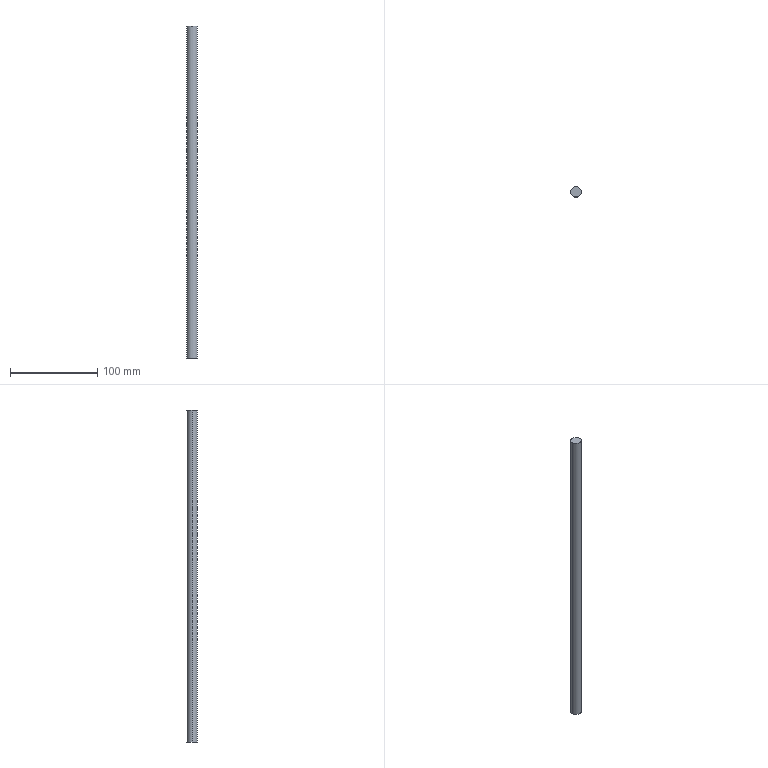Part | SolidWorks | features Extrusion 1 | 1 solid | 4 faces | box 12 x 12 x 380 mm | volume 42977 mm3 | cylinder 2 | plane 2 | commonest cylinder face diameters 12 x2
STEP:
#1=CARTESIAN_POINT('',(6.,0.,-190.));
#2=VERTEX_POINT('',#1);
#3=CARTESIAN_POINT('',(-6.,0.,-190.));
#4=VERTEX_POINT('',#3);
#5=CARTESIAN_POINT('',(0.,0.,-190.));
#6=DIRECTION('',(0.,0.,1.));
#7=DIRECTION('',(1.,0.,0.));
#8=AXIS2_PLACEMENT_3D('',#5,#6,#7);
#9=CIRCLE('',#8,6.);
#10=EDGE_CURVE('',#2,#4,#9,.T.);
#11=ORIENTED_EDGE('',*,*,#10,.T.);
#12=CARTESIAN_POINT('',(-6.,0.,190.));
#13=VERTEX_POINT('',#12);
#14=CARTESIAN_POINT('',(-6.,0.,-190.));
#15=DIRECTION('',(0.,0.,1.));
#16=VECTOR('',#15,1000.);
#17=LINE('',#14,#16);
#18=EDGE_CURVE('',#4,#13,#17,.T.);
#19=ORIENTED_EDGE('',*,*,#18,.T.);
#20=CARTESIAN_POINT('',(6.,0.,190.));
#21=VERTEX_POINT('',#20);
#22=CARTESIAN_POINT('',(0.,0.,190.));
#23=DIRECTION('',(0.,0.,1.));
#24=DIRECTION('',(1.,0.,0.));
#25=AXIS2_PLACEMENT_3D('',#22,#23,#24);
#26=CIRCLE('',#25,6.);
#27=EDGE_CURVE('',#21,#13,#26,.T.);
#28=ORIENTED_EDGE('',*,*,#27,.F.);
#29=CARTESIAN_POINT('',(6.,0.,-190.));
#30=DIRECTION('',(0.,0.,1.));
#31=VECTOR('',#30,1000.);
#32=LINE('',#29,#31);
#33=EDGE_CURVE('',#2,#21,#32,.T.);
#34=ORIENTED_EDGE('',*,*,#33,.F.);
#35=EDGE_LOOP('',(#11,#19,#28,#34));
#36=FACE_OUTER_BOUND('',#35,.T.);
#37=CARTESIAN_POINT('',(0.,0.,-190.));
#38=DIRECTION('',(0.,0.,1.));
#39=DIRECTION('',(1.,0.,0.));
#40=AXIS2_PLACEMENT_3D('',#37,#38,#39);
#41=CYLINDRICAL_SURFACE('',#40,6.);
#42=ADVANCED_FACE('',(#36),#41,.T.);
#43=ORIENTED_EDGE('',*,*,#18,.F.);
#44=CARTESIAN_POINT('',(0.,0.,-190.));
#45=DIRECTION('',(0.,0.,1.));
#46=DIRECTION('',(1.,0.,0.));
#47=AXIS2_PLACEMENT_3D('',#44,#45,#46);
#48=CIRCLE('',#47,6.);
#49=EDGE_CURVE('',#4,#2,#48,.T.);
#50=ORIENTED_EDGE('',*,*,#49,.T.);
#51=ORIENTED_EDGE('',*,*,#33,.T.);
#52=CARTESIAN_POINT('',(0.,0.,190.));
#53=DIRECTION('',(0.,0.,1.));
#54=DIRECTION('',(1.,0.,0.));
#55=AXIS2_PLACEMENT_3D('',#52,#53,#54);
#56=CIRCLE('',#55,6.);
#57=EDGE_CURVE('',#13,#21,#56,.T.);
#58=ORIENTED_EDGE('',*,*,#57,.F.);
#59=EDGE_LOOP('',(#43,#50,#51,#58));
#60=FACE_OUTER_BOUND('',#59,.T.);
#61=CARTESIAN_POINT('',(0.,0.,-190.));
#62=DIRECTION('',(0.,0.,1.));
#63=DIRECTION('',(1.,0.,0.));
#64=AXIS2_PLACEMENT_3D('',#61,#62,#63);
#65=CYLINDRICAL_SURFACE('',#64,6.);
#66=ADVANCED_FACE('',(#60),#65,.T.);
#67=ORIENTED_EDGE('',*,*,#10,.F.);
#68=ORIENTED_EDGE('',*,*,#49,.F.);
#69=EDGE_LOOP('',(#67,#68));
#70=FACE_OUTER_BOUND('',#69,.T.);
#71=CARTESIAN_POINT('',(0.,0.,-190.));
#72=DIRECTION('',(0.,0.,1.));
#73=DIRECTION('',(1.,0.,0.));
#74=AXIS2_PLACEMENT_3D('',#71,#72,#73);
#75=PLANE('',#74);
#76=ADVANCED_FACE('',(#70),#75,.F.);
#77=ORIENTED_EDGE('',*,*,#27,.T.);
#78=ORIENTED_EDGE('',*,*,#57,.T.);
#79=EDGE_LOOP('',(#77,#78));
#80=FACE_OUTER_BOUND('',#79,.T.);
#81=CARTESIAN_POINT('',(0.,0.,190.));
#82=DIRECTION('',(0.,0.,1.));
#83=DIRECTION('',(1.,0.,0.));
#84=AXIS2_PLACEMENT_3D('',#81,#82,#83);
#85=PLANE('',#84);
#86=ADVANCED_FACE('',(#80),#85,.T.);
#87=CLOSED_SHELL('',(#42,#66,#76,#86));
#88=MANIFOLD_SOLID_BREP('',#87);
#89=CARTESIAN_POINT('',(0.,0.,0.));
#90=DIRECTION('',(0.,0.,1.));
#91=DIRECTION('',(1.,0.,0.));
#92=AXIS2_PLACEMENT_3D('',#89,#90,#91);
#93=(LENGTH_UNIT()NAMED_UNIT(*)SI_UNIT(.MILLI.,.METRE.));
#94=UNCERTAINTY_MEASURE_WITH_UNIT(LENGTH_MEASURE(0.00001),#93,'','');
#95=(NAMED_UNIT(*)PLANE_ANGLE_UNIT()SI_UNIT($,.RADIAN.));
#96=(NAMED_UNIT(*)SI_UNIT($,.STERADIAN.)SOLID_ANGLE_UNIT());
#97=(GEOMETRIC_REPRESENTATION_CONTEXT(3)GLOBAL_UNCERTAINTY_ASSIGNED_CONTEXT((#94))GLOBAL_UNIT_ASSIGNED_CONTEXT((#93,#95,#96))REPRESENTATION_CONTEXT('',''));
#98=ADVANCED_BREP_SHAPE_REPRESENTATION('',(#88,#92),#97);